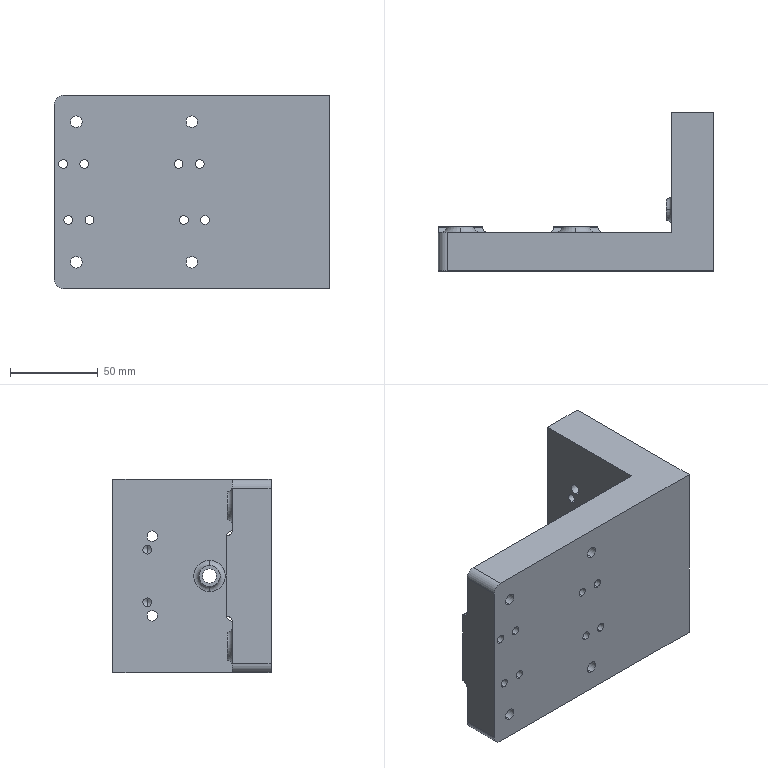Part | SolidWorks | features ICE 7, Fillet 2, Cut 1, Extrusion 1, HoleWzd 1 | 1 solid | 91 faces | box 156.771 x 90 x 110 mm | volume 550567 mm3 | cylinder 51 | plane 26 | torus 10 | cone 4 | commonest cylinder face diameters 5 x20 6 x17 6.647 x8 8 x2 10 x2 38 x2